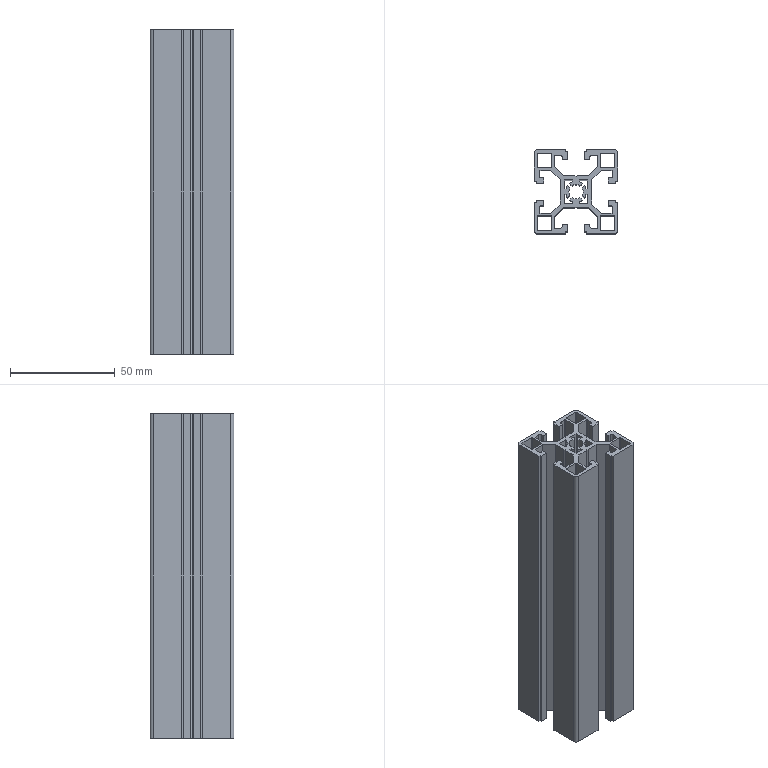Part | SolidWorks | features BaseBody 1, HoleWzd 1, MoveFace 1 | 1 solid | 179 faces | box 40 x 40 x 155 mm | volume 83065 mm3 | plane 130 | cylinder 49 | commonest cylinder face diameters 0.6 x24 2 x8 10 x8 6.8 x5 3 x4